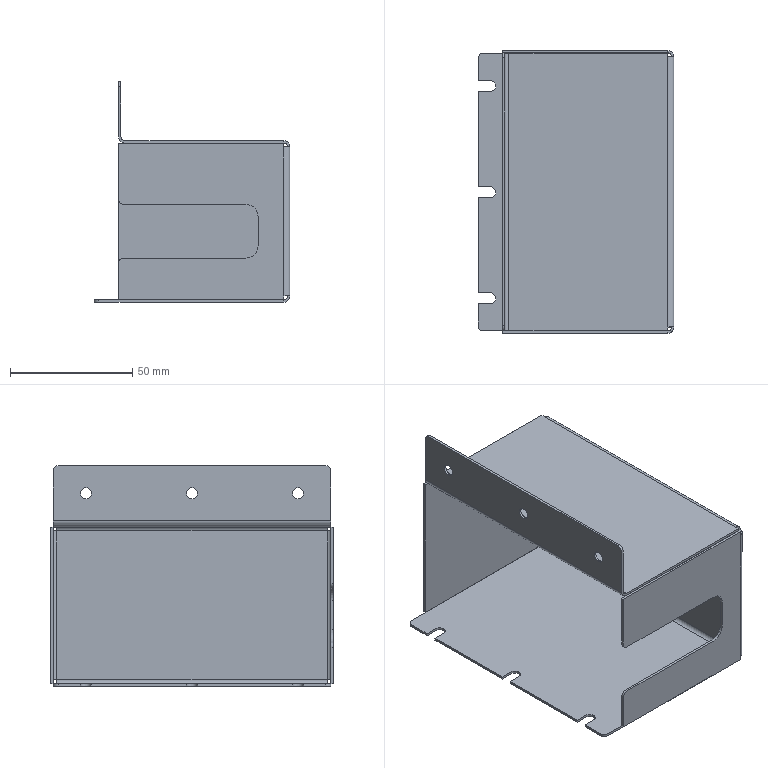Part | NX | 1 solid | 86 faces | box 80 x 115.5 x 90 mm | volume 34088 mm3 | plane 53 | cylinder 27 | cone 6 | commonest cylinder face diameters 4.5 x9 4 x6 3.2 x5 5.2 x5 10 x2